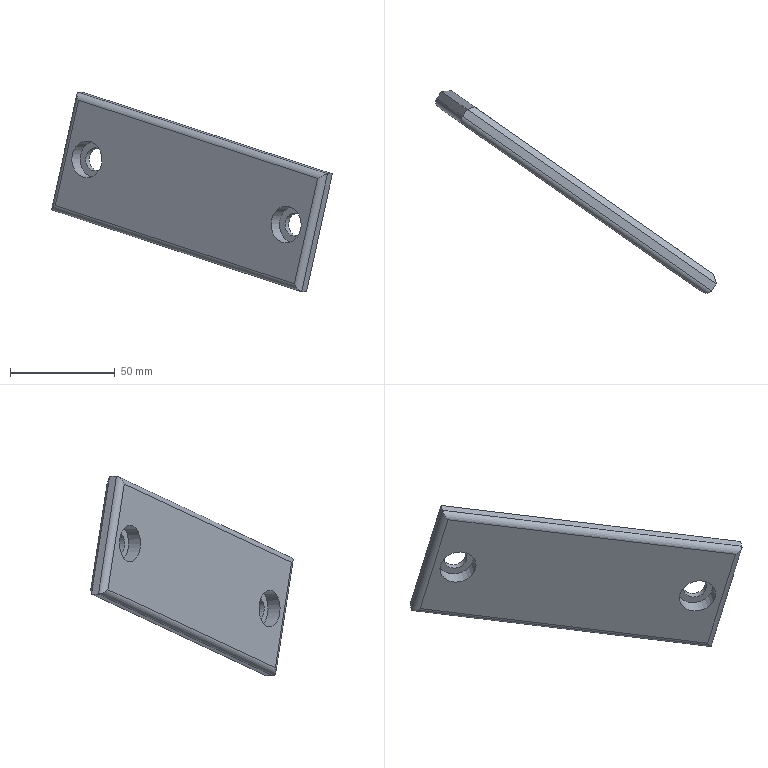Part | NX | features solid 2 | 1 solid | 20 faces | box 133.734 x 96.472 x 94.847 mm | volume 80433 mm3 | plane 12 | cylinder 8 | commonest cylinder face diameters 6 x4 11 x2 17.5 x2
STEP:
#1=CARTESIAN_POINT('',(-323.029,-70.461,-508.294));
#2=VERTEX_POINT('',#1);
#3=CARTESIAN_POINT('',(-325.323,-73.737,-508.294));
#4=VERTEX_POINT('',#3);
#5=CARTESIAN_POINT('',(-321.308,-68.003,-508.294));
#6=DIRECTION('',(-0.5736,-0.8192,0.));
#7=VECTOR('',#6,1000.);
#8=LINE('',#5,#7);
#9=EDGE_CURVE('',#2,#4,#8,.T.);
#10=ORIENTED_EDGE('',*,*,#9,.F.);
#11=CARTESIAN_POINT('',(-310.732,-79.071,-452.27));
#12=VERTEX_POINT('',#11);
#13=CARTESIAN_POINT('',(-308.93,-80.333,-444.06));
#14=DIRECTION('',(0.212,-0.1485,0.9659));
#15=VECTOR('',#14,1000.);
#16=LINE('',#13,#15);
#17=EDGE_CURVE('',#2,#12,#16,.T.);
#18=ORIENTED_EDGE('',*,*,#17,.T.);
#19=CARTESIAN_POINT('',(-313.027,-82.348,-452.27));
#20=VERTEX_POINT('',#19);
#21=CARTESIAN_POINT('',(-309.012,-76.614,-452.27));
#22=DIRECTION('',(-0.5736,-0.8192,0.));
#23=VECTOR('',#22,1000.);
#24=LINE('',#21,#23);
#25=EDGE_CURVE('',#12,#20,#24,.T.);
#26=ORIENTED_EDGE('',*,*,#25,.T.);
#27=CARTESIAN_POINT('',(-327.126,-72.476,-516.504));
#28=DIRECTION('',(-0.212,0.1485,-0.9659));
#29=VECTOR('',#28,1000.);
#30=LINE('',#27,#29);
#31=EDGE_CURVE('',#20,#4,#30,.T.);
#32=ORIENTED_EDGE('',*,*,#31,.T.);
#33=EDGE_LOOP('',(#10,#18,#26,#32));
#34=FACE_BOUND('',#33,.T.);
#35=CARTESIAN_POINT('',(-307.21,-77.875,-444.06));
#36=DIRECTION('',(-0.7912,0.554,0.2588));
#37=DIRECTION('',(0.212,-0.1485,0.9659));
#38=AXIS2_PLACEMENT_3D('',#35,#36,#37);
#39=PLANE('',#38);
#40=ADVANCED_FACE('',(#34),#39,.F.);
#41=CARTESIAN_POINT('',(-441.715,12.644,-469.471));
#42=VERTEX_POINT('',#41);
#43=CARTESIAN_POINT('',(-444.009,9.367,-469.471));
#44=VERTEX_POINT('',#43);
#45=CARTESIAN_POINT('',(-439.994,15.102,-469.471));
#46=DIRECTION('',(-0.5736,-0.8192,0.));
#47=VECTOR('',#46,1000.);
#48=LINE('',#45,#47);
#49=EDGE_CURVE('',#42,#44,#48,.T.);
#50=ORIENTED_EDGE('',*,*,#49,.F.);
#51=CARTESIAN_POINT('',(-382.372,-28.908,-488.882));
#52=DIRECTION('',(0.7912,-0.554,-0.2588));
#53=VECTOR('',#52,1000.);
#54=LINE('',#51,#53);
#55=EDGE_CURVE('',#42,#2,#54,.T.);
#56=ORIENTED_EDGE('',*,*,#55,.T.);
#57=ORIENTED_EDGE('',*,*,#9,.T.);
#58=CARTESIAN_POINT('',(-444.009,9.367,-469.471));
#59=DIRECTION('',(-0.7912,0.554,0.2588));
#60=VECTOR('',#59,1000.);
#61=LINE('',#58,#60);
#62=EDGE_CURVE('',#4,#44,#61,.T.);
#63=ORIENTED_EDGE('',*,*,#62,.T.);
#64=EDGE_LOOP('',(#50,#56,#57,#63));
#65=FACE_BOUND('',#64,.T.);
#66=CARTESIAN_POINT('',(-380.651,-26.451,-488.882));
#67=DIRECTION('',(0.212,-0.1485,0.9659));
#68=DIRECTION('',(0.5736,0.8192,0.));
#69=AXIS2_PLACEMENT_3D('',#66,#67,#68);
#70=PLANE('',#69);
#71=ADVANCED_FACE('',(#65),#70,.F.);
#72=CARTESIAN_POINT('',(-429.418,4.034,-413.447));
#73=VERTEX_POINT('',#72);
#74=CARTESIAN_POINT('',(-431.713,0.7572,-413.447));
#75=VERTEX_POINT('',#74);
#76=CARTESIAN_POINT('',(-427.698,6.491,-413.447));
#77=DIRECTION('',(-0.5736,-0.8192,0.));
#78=VECTOR('',#77,1000.);
#79=LINE('',#76,#78);
#80=EDGE_CURVE('',#73,#75,#79,.T.);
#81=ORIENTED_EDGE('',*,*,#80,.F.);
#82=CARTESIAN_POINT('',(-443.517,13.906,-477.681));
#83=DIRECTION('',(-0.212,0.1485,-0.9659));
#84=VECTOR('',#83,1000.);
#85=LINE('',#82,#84);
#86=EDGE_CURVE('',#73,#42,#85,.T.);
#87=ORIENTED_EDGE('',*,*,#86,.T.);
#88=ORIENTED_EDGE('',*,*,#49,.T.);
#89=CARTESIAN_POINT('',(-429.911,-0.5046,-405.237));
#90=DIRECTION('',(0.212,-0.1485,0.9659));
#91=VECTOR('',#90,1000.);
#92=LINE('',#89,#91);
#93=EDGE_CURVE('',#44,#75,#92,.T.);
#94=ORIENTED_EDGE('',*,*,#93,.T.);
#95=EDGE_LOOP('',(#81,#87,#88,#94));
#96=FACE_BOUND('',#95,.T.);
#97=CARTESIAN_POINT('',(-441.797,16.363,-477.681));
#98=DIRECTION('',(0.7912,-0.554,-0.2588));
#99=DIRECTION('',(0.5736,0.8192,0.));
#100=AXIS2_PLACEMENT_3D('',#97,#98,#99);
#101=PLANE('',#100);
#102=ADVANCED_FACE('',(#96),#101,.F.);
#103=ORIENTED_EDGE('',*,*,#25,.F.);
#104=CARTESIAN_POINT('',(-409.637,-9.817,-419.918));
#105=DIRECTION('',(-0.7912,0.554,0.2588));
#106=VECTOR('',#105,1000.);
#107=LINE('',#104,#106);
#108=EDGE_CURVE('',#12,#73,#107,.T.);
#109=ORIENTED_EDGE('',*,*,#108,.T.);
#110=ORIENTED_EDGE('',*,*,#80,.T.);
#111=CARTESIAN_POINT('',(-352.589,-54.646,-439.329));
#112=DIRECTION('',(0.7912,-0.554,-0.2588));
#113=VECTOR('',#112,1000.);
#114=LINE('',#111,#113);
#115=EDGE_CURVE('',#75,#20,#114,.T.);
#116=ORIENTED_EDGE('',*,*,#115,.T.);
#117=EDGE_LOOP('',(#103,#109,#110,#116));
#118=FACE_BOUND('',#117,.T.);
#119=CARTESIAN_POINT('',(-407.917,-7.36,-419.918));
#120=DIRECTION('',(-0.212,0.1485,-0.9659));
#121=DIRECTION('',(-0.7912,0.554,0.2588));
#122=AXIS2_PLACEMENT_3D('',#119,#120,#121);
#123=PLANE('',#122);
#124=ADVANCED_FACE('',(#118),#123,.F.);
#125=CARTESIAN_POINT('',(-323.046,-66.787,-504.619));
#126=VERTEX_POINT('',#125);
#127=CARTESIAN_POINT('',(-436.985,12.994,-467.349));
#128=VERTEX_POINT('',#127);
#129=CARTESIAN_POINT('',(-380.015,-26.896,-485.984));
#130=DIRECTION('',(-0.7912,0.554,0.2588));
#131=VECTOR('',#130,1000.);
#132=LINE('',#129,#131);
#133=EDGE_CURVE('',#126,#128,#132,.T.);
#134=ORIENTED_EDGE('',*,*,#133,.T.);
#135=CARTESIAN_POINT('',(-425.96,5.275,-417.121));
#136=VERTEX_POINT('',#135);
#137=CARTESIAN_POINT('',(-423.522,3.567,-406.013));
#138=DIRECTION('',(0.212,-0.1485,0.9659));
#139=VECTOR('',#138,1000.);
#140=LINE('',#137,#139);
#141=EDGE_CURVE('',#128,#136,#140,.T.);
#142=ORIENTED_EDGE('',*,*,#141,.T.);
#143=CARTESIAN_POINT('',(-312.021,-74.506,-454.391));
#144=VERTEX_POINT('',#143);
#145=CARTESIAN_POINT('',(-368.991,-34.616,-435.756));
#146=DIRECTION('',(0.7912,-0.554,-0.2588));
#147=VECTOR('',#146,1000.);
#148=LINE('',#145,#147);
#149=EDGE_CURVE('',#136,#144,#148,.T.);
#150=ORIENTED_EDGE('',*,*,#149,.T.);
#151=CARTESIAN_POINT('',(-309.583,-76.213,-443.283));
#152=DIRECTION('',(-0.212,0.1485,-0.9659));
#153=VECTOR('',#152,1000.);
#154=LINE('',#151,#153);
#155=EDGE_CURVE('',#144,#126,#154,.T.);
#156=ORIENTED_EDGE('',*,*,#155,.T.);
#157=EDGE_LOOP('',(#134,#142,#150,#156));
#158=FACE_BOUND('',#157,.T.);
#159=CARTESIAN_POINT('',(-417.626,-0.5613,-446.765));
#160=VERTEX_POINT('',#159);
#161=CARTESIAN_POINT('',(-421.977,2.486,-445.341));
#162=DIRECTION('',(-0.5736,-0.8192,0.));
#163=DIRECTION('',(0.7912,-0.554,-0.2588));
#164=AXIS2_PLACEMENT_3D('',#161,#162,#163);
#165=CIRCLE('',#164,5.5);
#166=EDGE_CURVE('',#160,#160,#165,.T.);
#167=ORIENTED_EDGE('',*,*,#166,.T.);
#168=EDGE_LOOP('',(#167));
#169=FACE_BOUND('',#168,.T.);
#170=CARTESIAN_POINT('',(-322.677,-67.045,-477.823));
#171=VERTEX_POINT('',#170);
#172=CARTESIAN_POINT('',(-327.029,-63.998,-476.4));
#173=DIRECTION('',(-0.5736,-0.8192,0.));
#174=DIRECTION('',(0.7912,-0.554,-0.2588));
#175=AXIS2_PLACEMENT_3D('',#172,#173,#174);
#176=CIRCLE('',#175,5.5);
#177=EDGE_CURVE('',#171,#171,#176,.T.);
#178=ORIENTED_EDGE('',*,*,#177,.T.);
#179=EDGE_LOOP('',(#178));
#180=FACE_BOUND('',#179,.T.);
#181=CARTESIAN_POINT('',(-366.553,-36.323,-424.648));
#182=DIRECTION('',(-0.5736,-0.8192,0.));
#183=DIRECTION('',(0.7912,-0.554,-0.2588));
#184=AXIS2_PLACEMENT_3D('',#181,#182,#183);
#185=PLANE('',#184);
#186=ADVANCED_FACE('',(#158,#169,#180),#185,.F.);
#187=CARTESIAN_POINT('',(-328.782,-74.978,-504.619));
#188=VERTEX_POINT('',#187);
#189=CARTESIAN_POINT('',(-317.757,-82.698,-454.391));
#190=VERTEX_POINT('',#189);
#191=CARTESIAN_POINT('',(-315.319,-84.405,-443.283));
#192=DIRECTION('',(-0.212,0.1485,-0.9659));
#193=VECTOR('',#192,1000.);
#194=LINE('',#191,#193);
#195=EDGE_CURVE('',#188,#190,#194,.F.);
#196=ORIENTED_EDGE('',*,*,#195,.T.);
#197=CARTESIAN_POINT('',(-431.696,-2.917,-417.121));
#198=VERTEX_POINT('',#197);
#199=CARTESIAN_POINT('',(-414.289,-15.106,-422.815));
#200=DIRECTION('',(0.7912,-0.554,-0.2588));
#201=VECTOR('',#200,1000.);
#202=LINE('',#199,#201);
#203=EDGE_CURVE('',#190,#198,#202,.F.);
#204=ORIENTED_EDGE('',*,*,#203,.T.);
#205=CARTESIAN_POINT('',(-442.72,4.803,-467.349));
#206=VERTEX_POINT('',#205);
#207=CARTESIAN_POINT('',(-445.159,6.51,-478.458));
#208=DIRECTION('',(0.212,-0.1485,0.9659));
#209=VECTOR('',#208,1000.);
#210=LINE('',#207,#209);
#211=EDGE_CURVE('',#198,#206,#210,.F.);
#212=ORIENTED_EDGE('',*,*,#211,.T.);
#213=CARTESIAN_POINT('',(-385.751,-35.088,-485.984));
#214=DIRECTION('',(-0.7912,0.554,0.2588));
#215=VECTOR('',#214,1000.);
#216=LINE('',#213,#215);
#217=EDGE_CURVE('',#206,#188,#216,.F.);
#218=ORIENTED_EDGE('',*,*,#217,.T.);
#219=EDGE_LOOP('',(#196,#204,#212,#218));
#220=FACE_BOUND('',#219,.T.);
#221=CARTESIAN_POINT('',(-434.637,-0.8578,-443.077));
#222=VERTEX_POINT('',#221);
#223=CARTESIAN_POINT('',(-427.713,-5.706,-445.341));
#224=DIRECTION('',(0.5736,0.8192,0.));
#225=DIRECTION('',(-0.7912,0.554,0.2588));
#226=AXIS2_PLACEMENT_3D('',#223,#224,#225);
#227=CIRCLE('',#226,8.75);
#228=EDGE_CURVE('',#222,#222,#227,.T.);
#229=ORIENTED_EDGE('',*,*,#228,.T.);
#230=EDGE_LOOP('',(#229));
#231=FACE_BOUND('',#230,.T.);
#232=CARTESIAN_POINT('',(-339.688,-67.342,-474.135));
#233=VERTEX_POINT('',#232);
#234=CARTESIAN_POINT('',(-332.764,-72.189,-476.4));
#235=DIRECTION('',(0.5736,0.8192,0.));
#236=DIRECTION('',(-0.7912,0.554,0.2588));
#237=AXIS2_PLACEMENT_3D('',#234,#235,#236);
#238=CIRCLE('',#237,8.75);
#239=EDGE_CURVE('',#233,#233,#238,.T.);
#240=ORIENTED_EDGE('',*,*,#239,.T.);
#241=EDGE_LOOP('',(#240));
#242=FACE_BOUND('',#241,.T.);
#243=CARTESIAN_POINT('',(-372.288,-44.515,-424.648));
#244=DIRECTION('',(-0.5736,-0.8192,0.));
#245=DIRECTION('',(0.7912,-0.554,-0.2588));
#246=AXIS2_PLACEMENT_3D('',#243,#244,#245);
#247=PLANE('',#246);
#248=ADVANCED_FACE('',(#220,#231,#242),#247,.T.);
#249=CARTESIAN_POINT('',(-332.651,-63.723,-473.65));
#250=VERTEX_POINT('',#249);
#251=CARTESIAN_POINT('',(-328.749,-66.455,-476.4));
#252=DIRECTION('',(-0.5736,-0.8192,0.));
#253=DIRECTION('',(-0.7094,0.4967,0.5));
#254=AXIS2_PLACEMENT_3D('',#251,#252,#253);
#255=CIRCLE('',#254,5.5);
#256=EDGE_CURVE('',#250,#250,#255,.F.);
#257=ORIENTED_EDGE('',*,*,#256,.F.);
#258=EDGE_LOOP('',(#257));
#259=FACE_BOUND('',#258,.T.);
#260=ORIENTED_EDGE('',*,*,#177,.F.);
#261=EDGE_LOOP('',(#260));
#262=FACE_BOUND('',#261,.T.);
#263=CARTESIAN_POINT('',(-309.821,-39.423,-476.4));
#264=DIRECTION('',(0.5736,0.8192,0.));
#265=DIRECTION('',(-0.7912,0.554,0.2588));
#266=AXIS2_PLACEMENT_3D('',#263,#264,#265);
#267=CYLINDRICAL_SURFACE('',#266,5.5);
#268=ADVANCED_FACE('',(#259,#262),#267,.F.);
#269=ORIENTED_EDGE('',*,*,#256,.T.);
#270=EDGE_LOOP('',(#269));
#271=FACE_BOUND('',#270,.T.);
#272=CARTESIAN_POINT('',(-334.957,-62.109,-472.025));
#273=VERTEX_POINT('',#272);
#274=CARTESIAN_POINT('',(-328.749,-66.455,-476.4));
#275=DIRECTION('',(-0.5736,-0.8192,0.));
#276=DIRECTION('',(-0.7094,0.4967,0.5));
#277=AXIS2_PLACEMENT_3D('',#274,#275,#276);
#278=CIRCLE('',#277,8.75);
#279=EDGE_CURVE('',#273,#273,#278,.F.);
#280=ORIENTED_EDGE('',*,*,#279,.F.);
#281=EDGE_LOOP('',(#280));
#282=FACE_BOUND('',#281,.T.);
#283=CARTESIAN_POINT('',(-328.749,-66.455,-476.4));
#284=DIRECTION('',(0.5736,0.8192,0.));
#285=DIRECTION('',(-0.7912,0.554,0.2588));
#286=AXIS2_PLACEMENT_3D('',#283,#284,#285);
#287=PLANE('',#286);
#288=ADVANCED_FACE('',(#271,#282),#287,.F.);
#289=ORIENTED_EDGE('',*,*,#279,.T.);
#290=EDGE_LOOP('',(#289));
#291=FACE_BOUND('',#290,.T.);
#292=ORIENTED_EDGE('',*,*,#239,.F.);
#293=EDGE_LOOP('',(#292));
#294=FACE_BOUND('',#293,.T.);
#295=CARTESIAN_POINT('',(-338.5,-80.381,-476.4));
#296=DIRECTION('',(0.5736,0.8192,0.));
#297=DIRECTION('',(-0.7912,0.554,0.2588));
#298=AXIS2_PLACEMENT_3D('',#295,#296,#297);
#299=CYLINDRICAL_SURFACE('',#298,8.75);
#300=ADVANCED_FACE('',(#291,#294),#299,.F.);
#301=CARTESIAN_POINT('',(-427.6,2.76,-442.591));
#302=VERTEX_POINT('',#301);
#303=CARTESIAN_POINT('',(-423.698,0.02846,-445.341));
#304=DIRECTION('',(-0.5736,-0.8192,0.));
#305=DIRECTION('',(-0.7094,0.4967,0.5));
#306=AXIS2_PLACEMENT_3D('',#303,#304,#305);
#307=CIRCLE('',#306,5.5);
#308=EDGE_CURVE('',#302,#302,#307,.F.);
#309=ORIENTED_EDGE('',*,*,#308,.F.);
#310=EDGE_LOOP('',(#309));
#311=FACE_BOUND('',#310,.T.);
#312=ORIENTED_EDGE('',*,*,#166,.F.);
#313=EDGE_LOOP('',(#312));
#314=FACE_BOUND('',#313,.T.);
#315=CARTESIAN_POINT('',(-404.77,27.06,-445.341));
#316=DIRECTION('',(0.5736,0.8192,0.));
#317=DIRECTION('',(-0.7912,0.554,0.2588));
#318=AXIS2_PLACEMENT_3D('',#315,#316,#317);
#319=CYLINDRICAL_SURFACE('',#318,5.5);
#320=ADVANCED_FACE('',(#311,#314),#319,.F.);
#321=ORIENTED_EDGE('',*,*,#308,.T.);
#322=EDGE_LOOP('',(#321));
#323=FACE_BOUND('',#322,.T.);
#324=CARTESIAN_POINT('',(-429.906,4.375,-440.966));
#325=VERTEX_POINT('',#324);
#326=CARTESIAN_POINT('',(-423.698,0.02846,-445.341));
#327=DIRECTION('',(-0.5736,-0.8192,0.));
#328=DIRECTION('',(-0.7094,0.4967,0.5));
#329=AXIS2_PLACEMENT_3D('',#326,#327,#328);
#330=CIRCLE('',#329,8.75);
#331=EDGE_CURVE('',#325,#325,#330,.F.);
#332=ORIENTED_EDGE('',*,*,#331,.F.);
#333=EDGE_LOOP('',(#332));
#334=FACE_BOUND('',#333,.T.);
#335=CARTESIAN_POINT('',(-423.698,0.02846,-445.341));
#336=DIRECTION('',(0.5736,0.8192,0.));
#337=DIRECTION('',(-0.7912,0.554,0.2588));
#338=AXIS2_PLACEMENT_3D('',#335,#336,#337);
#339=PLANE('',#338);
#340=ADVANCED_FACE('',(#323,#334),#339,.F.);
#341=ORIENTED_EDGE('',*,*,#331,.T.);
#342=EDGE_LOOP('',(#341));
#343=FACE_BOUND('',#342,.T.);
#344=ORIENTED_EDGE('',*,*,#228,.F.);
#345=EDGE_LOOP('',(#344));
#346=FACE_BOUND('',#345,.T.);
#347=CARTESIAN_POINT('',(-433.449,-13.897,-445.341));
#348=DIRECTION('',(0.5736,0.8192,0.));
#349=DIRECTION('',(-0.7912,0.554,0.2588));
#350=AXIS2_PLACEMENT_3D('',#347,#348,#349);
#351=CYLINDRICAL_SURFACE('',#350,8.75);
#352=ADVANCED_FACE('',(#343,#346),#351,.F.);
#353=CARTESIAN_POINT('',(-327.061,-72.521,-504.619));
#354=DIRECTION('',(0.7094,-0.4967,0.5));
#355=DIRECTION('',(-0.4096,0.2868,0.866));
#356=AXIS2_PLACEMENT_3D('',#353,#354,#355);
#357=ELLIPSE('',#356,4.243,3.);
#358=EDGE_CURVE('',#188,#4,#357,.T.);
#359=ORIENTED_EDGE('',*,*,#358,.F.);
#360=ORIENTED_EDGE('',*,*,#217,.F.);
#361=CARTESIAN_POINT('',(-441.,7.26,-467.349));
#362=DIRECTION('',(0.4096,-0.2868,-0.866));
#363=DIRECTION('',(0.7094,-0.4967,0.5));
#364=AXIS2_PLACEMENT_3D('',#361,#362,#363);
#365=ELLIPSE('',#364,4.243,3.);
#366=EDGE_CURVE('',#44,#206,#365,.F.);
#367=ORIENTED_EDGE('',*,*,#366,.F.);
#368=ORIENTED_EDGE('',*,*,#62,.F.);
#369=EDGE_LOOP('',(#359,#360,#367,#368));
#370=FACE_BOUND('',#369,.T.);
#371=CARTESIAN_POINT('',(-384.03,-32.63,-485.984));
#372=DIRECTION('',(0.7912,-0.554,-0.2588));
#373=DIRECTION('',(0.5736,0.8192,0.));
#374=AXIS2_PLACEMENT_3D('',#371,#372,#373);
#375=CYLINDRICAL_SURFACE('',#374,3.);
#376=ADVANCED_FACE('',(#370),#375,.T.);
#377=ORIENTED_EDGE('',*,*,#366,.T.);
#378=ORIENTED_EDGE('',*,*,#211,.F.);
#379=CARTESIAN_POINT('',(-429.975,-0.4595,-417.121));
#380=DIRECTION('',(-0.7094,0.4967,-0.5));
#381=DIRECTION('',(0.4096,-0.2868,-0.866));
#382=AXIS2_PLACEMENT_3D('',#379,#380,#381);
#383=ELLIPSE('',#382,4.243,3.);
#384=EDGE_CURVE('',#75,#198,#383,.F.);
#385=ORIENTED_EDGE('',*,*,#384,.F.);
#386=ORIENTED_EDGE('',*,*,#93,.F.);
#387=EDGE_LOOP('',(#377,#378,#385,#386));
#388=FACE_BOUND('',#387,.T.);
#389=CARTESIAN_POINT('',(-443.438,8.967,-478.458));
#390=DIRECTION('',(-0.212,0.1485,-0.9659));
#391=DIRECTION('',(-0.5736,-0.8192,0.));
#392=AXIS2_PLACEMENT_3D('',#389,#390,#391);
#393=CYLINDRICAL_SURFACE('',#392,3.);
#394=ADVANCED_FACE('',(#388),#393,.T.);
#395=ORIENTED_EDGE('',*,*,#358,.T.);
#396=ORIENTED_EDGE('',*,*,#31,.F.);
#397=CARTESIAN_POINT('',(-316.037,-80.24,-454.391));
#398=DIRECTION('',(-0.4096,0.2868,0.866));
#399=DIRECTION('',(-0.7094,0.4967,-0.5));
#400=AXIS2_PLACEMENT_3D('',#397,#398,#399);
#401=ELLIPSE('',#400,4.243,3.);
#402=EDGE_CURVE('',#190,#20,#401,.T.);
#403=ORIENTED_EDGE('',*,*,#402,.F.);
#404=ORIENTED_EDGE('',*,*,#195,.F.);
#405=EDGE_LOOP('',(#395,#396,#403,#404));
#406=FACE_BOUND('',#405,.T.);
#407=CARTESIAN_POINT('',(-313.598,-81.947,-443.283));
#408=DIRECTION('',(0.212,-0.1485,0.9659));
#409=DIRECTION('',(0.7912,-0.554,-0.2588));
#410=AXIS2_PLACEMENT_3D('',#407,#408,#409);
#411=CYLINDRICAL_SURFACE('',#410,3.);
#412=ADVANCED_FACE('',(#406),#411,.T.);
#413=ORIENTED_EDGE('',*,*,#384,.T.);
#414=ORIENTED_EDGE('',*,*,#203,.F.);
#415=ORIENTED_EDGE('',*,*,#402,.T.);
#416=ORIENTED_EDGE('',*,*,#115,.F.);
#417=EDGE_LOOP('',(#413,#414,#415,#416));
#418=FACE_BOUND('',#417,.T.);
#419=CARTESIAN_POINT('',(-412.568,-12.648,-422.815));
#420=DIRECTION('',(-0.7912,0.554,0.2588));
#421=DIRECTION('',(0.212,-0.1485,0.9659));
#422=AXIS2_PLACEMENT_3D('',#419,#420,#421);
#423=CYLINDRICAL_SURFACE('',#422,3.);
#424=ADVANCED_FACE('',(#418),#423,.T.);
#425=CARTESIAN_POINT('',(-311.592,-76.028,-453.684));
#426=DIRECTION('',(-0.2481,0.8785,-0.4082));
#427=VECTOR('',#426,1000.);
#428=LINE('',#425,#427);
#429=EDGE_CURVE('',#12,#144,#428,.T.);
#430=ORIENTED_EDGE('',*,*,#429,.F.);
#431=ORIENTED_EDGE('',*,*,#17,.F.);
#432=CARTESIAN_POINT('',(-323.182,-37.393,-475.226));
#433=DIRECTION('',(-0.003263,0.7071,0.7071));
#434=VECTOR('',#433,1000.);
#435=LINE('',#432,#434);
#436=EDGE_CURVE('',#126,#2,#435,.F.);
#437=ORIENTED_EDGE('',*,*,#436,.F.);
#438=ORIENTED_EDGE('',*,*,#155,.F.);
#439=EDGE_LOOP('',(#430,#431,#437,#438));
#440=FACE_BOUND('',#439,.T.);
#441=CARTESIAN_POINT('',(-309.583,-76.213,-443.283));
#442=DIRECTION('',(-0.9651,-0.1875,0.183));
#443=DIRECTION('',(0.1539,-0.971,-0.183));
#444=AXIS2_PLACEMENT_3D('',#441,#442,#443);
#445=PLANE('',#444);
#446=ADVANCED_FACE('',(#440),#445,.F.);
#447=ORIENTED_EDGE('',*,*,#436,.T.);
#448=ORIENTED_EDGE('',*,*,#55,.F.);
#449=CARTESIAN_POINT('',(-399.141,15.794,-450.379));
#450=DIRECTION('',(0.9104,0.06736,0.4082));
#451=VECTOR('',#450,1000.);
#452=LINE('',#449,#451);
#453=EDGE_CURVE('',#128,#42,#452,.F.);
#454=ORIENTED_EDGE('',*,*,#453,.F.);
#455=ORIENTED_EDGE('',*,*,#133,.F.);
#456=EDGE_LOOP('',(#447,#448,#454,#455));
#457=FACE_BOUND('',#456,.T.);
#458=CARTESIAN_POINT('',(-380.015,-26.896,-485.984));
#459=DIRECTION('',(-0.2557,-0.6842,0.683));
#460=DIRECTION('',(0.5555,0.4743,0.683));
#461=AXIS2_PLACEMENT_3D('',#458,#459,#460);
#462=PLANE('',#461);
#463=ADVANCED_FACE('',(#457),#462,.F.);
#464=ORIENTED_EDGE('',*,*,#429,.T.);
#465=ORIENTED_EDGE('',*,*,#149,.F.);
#466=CARTESIAN_POINT('',(-398.293,15.2,-446.515));
#467=DIRECTION('',(-0.6656,-0.2388,0.7071));
#468=VECTOR('',#467,1000.);
#469=LINE('',#466,#468);
#470=EDGE_CURVE('',#73,#136,#469,.F.);
#471=ORIENTED_EDGE('',*,*,#470,.F.);
#472=ORIENTED_EDGE('',*,*,#108,.F.);
#473=EDGE_LOOP('',(#464,#465,#471,#472));
#474=FACE_BOUND('',#473,.T.);
#475=CARTESIAN_POINT('',(-368.991,-34.616,-435.756));
#476=DIRECTION('',(-0.5555,-0.4743,-0.683));
#477=DIRECTION('',(-0.2557,-0.6842,0.683));
#478=AXIS2_PLACEMENT_3D('',#475,#476,#477);
#479=PLANE('',#478);
#480=ADVANCED_FACE('',(#474),#479,.F.);
#481=ORIENTED_EDGE('',*,*,#453,.T.);
#482=ORIENTED_EDGE('',*,*,#86,.F.);
#483=ORIENTED_EDGE('',*,*,#470,.T.);
#484=ORIENTED_EDGE('',*,*,#141,.F.);
#485=EDGE_LOOP('',(#481,#482,#483,#484));
#486=FACE_BOUND('',#485,.T.);
#487=CARTESIAN_POINT('',(-423.522,3.567,-406.013));
#488=DIRECTION('',(0.1539,-0.971,-0.183));
#489=DIRECTION('',(0.9651,0.1875,-0.183));
#490=AXIS2_PLACEMENT_3D('',#487,#488,#489);
#491=PLANE('',#490);
#492=ADVANCED_FACE('',(#486),#491,.F.);
#493=CLOSED_SHELL('',(#40,#71,#102,#124,#186,#248,#268,#288,#300,#320,#340,#352,#376,#394,#412,#424,#446,#463,#480,#492));
#494=MANIFOLD_SOLID_BREP('',#493);
#495=(LENGTH_UNIT()NAMED_UNIT(*)SI_UNIT(.MILLI.,.METRE.));
#496=UNCERTAINTY_MEASURE_WITH_UNIT(LENGTH_MEASURE(0.00001),#495,'','');
#497=(NAMED_UNIT(*)PLANE_ANGLE_UNIT()SI_UNIT($,.RADIAN.));
#498=(NAMED_UNIT(*)SI_UNIT($,.STERADIAN.)SOLID_ANGLE_UNIT());
#499=(GEOMETRIC_REPRESENTATION_CONTEXT(3)GLOBAL_UNCERTAINTY_ASSIGNED_CONTEXT((#496))GLOBAL_UNIT_ASSIGNED_CONTEXT((#495,#497,#498))REPRESENTATION_CONTEXT('',''));
#500=ADVANCED_BREP_SHAPE_REPRESENTATION('',(#494),#499);